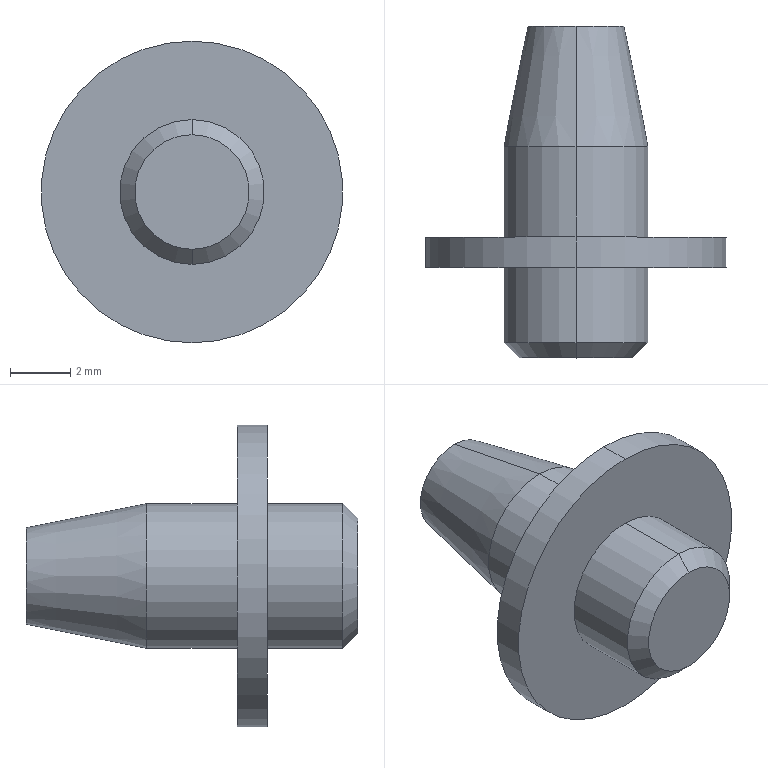Part | STEP file | TYLJ-BJ-007 Pin(1mm thick)-dddeger | 1 solid | 14 faces | box 10 x 11 x 10 mm | volume 236.295 mm3 | cylinder 6 | cone 4 | plane 4 | commonest cylinder face diameters 4.8 x4 10 x2
STEP:
#1=CARTESIAN_POINT('',(0.,0.,0.));
#2=DIRECTION('',(0.,0.,1.));
#3=DIRECTION('',(1.,0.,0.));
#4=AXIS2_PLACEMENT_3D('',#1,#2,#3);
#5=CARTESIAN_POINT('',(0.,0.,-1.9));
#6=VERTEX_POINT('',#5);
#7=CARTESIAN_POINT('',(0.,0.,1.9));
#8=VERTEX_POINT('',#7);
#9=CARTESIAN_POINT('',(0.,0.,0.));
#10=DIRECTION('',(0.,-1.,0.));
#11=DIRECTION('',(0.,0.,-1.));
#12=AXIS2_PLACEMENT_3D('',#9,#10,#11);
#13=CIRCLE('',#12,1.9);
#14=CARTESIAN_POINT('',(0.,0.,0.));
#15=DIRECTION('',(0.,1.,0.));
#16=DIRECTION('',(0.,0.,1.));
#17=AXIS2_PLACEMENT_3D('',#14,#15,#16);
#18=CONICAL_SURFACE('',#17,1.9,0.7854);
#19=CARTESIAN_POINT('',(3.142,0.));
#20=DIRECTION('',(-1.,0.));
#21=VECTOR('',#20,1.);
#22=LINE('',#19,#21);
#23=(GEOMETRIC_REPRESENTATION_CONTEXT(2)PARAMETRIC_REPRESENTATION_CONTEXT()REPRESENTATION_CONTEXT('',''));
#24=DEFINITIONAL_REPRESENTATION('',(#22),#23);
#25=PCURVE('',#18,#24);
#26=CARTESIAN_POINT('',(0.,0.,0.));
#27=DIRECTION('',(0.,-1.,0.));
#28=DIRECTION('',(0.,0.,-1.));
#29=AXIS2_PLACEMENT_3D('',#26,#27,#28);
#30=PLANE('',#29);
#31=CARTESIAN_POINT('',(0.,0.));
#32=DIRECTION('',(1.,0.));
#33=AXIS2_PLACEMENT_2D('',#31,#32);
#34=CIRCLE('',#33,1.9);
#35=(GEOMETRIC_REPRESENTATION_CONTEXT(2)PARAMETRIC_REPRESENTATION_CONTEXT()REPRESENTATION_CONTEXT('',''));
#36=DEFINITIONAL_REPRESENTATION('',(#34),#35);
#37=PCURVE('',#30,#36);
#38=SURFACE_CURVE('',#13,(#25,#37),.PCURVE_S1.);
#39=EDGE_CURVE('',#6,#8,#38,.T.);
#40=ORIENTED_EDGE('',*,*,#39,.F.);
#41=CARTESIAN_POINT('',(0.,0.5,-2.4));
#42=VERTEX_POINT('',#41);
#43=CARTESIAN_POINT('',(0.,0.,-1.9));
#44=DIRECTION('',(0.,0.7071,-0.7071));
#45=VECTOR('',#44,1.);
#46=LINE('',#43,#45);
#47=CARTESIAN_POINT('',(3.142,0.));
#48=DIRECTION('',(0.,1.));
#49=VECTOR('',#48,1.);
#50=LINE('',#47,#49);
#51=(GEOMETRIC_REPRESENTATION_CONTEXT(2)PARAMETRIC_REPRESENTATION_CONTEXT()REPRESENTATION_CONTEXT('',''));
#52=DEFINITIONAL_REPRESENTATION('',(#50),#51);
#53=PCURVE('',#18,#52);
#54=CARTESIAN_POINT('',(0.,0.,0.));
#55=DIRECTION('',(0.,1.,0.));
#56=DIRECTION('',(0.,0.,1.));
#57=AXIS2_PLACEMENT_3D('',#54,#55,#56);
#58=CONICAL_SURFACE('',#57,1.9,0.7854);
#59=CARTESIAN_POINT('',(3.142,0.));
#60=DIRECTION('',(0.,1.));
#61=VECTOR('',#60,1.);
#62=LINE('',#59,#61);
#63=(GEOMETRIC_REPRESENTATION_CONTEXT(2)PARAMETRIC_REPRESENTATION_CONTEXT()REPRESENTATION_CONTEXT('',''));
#64=DEFINITIONAL_REPRESENTATION('',(#62),#63);
#65=PCURVE('',#58,#64);
#66=SURFACE_CURVE('',#46,(#53,#65),.PCURVE_S1.);
#67=EDGE_CURVE('',#6,#42,#66,.T.);
#68=ORIENTED_EDGE('',*,*,#67,.T.);
#69=CARTESIAN_POINT('',(0.,0.5,2.4));
#70=VERTEX_POINT('',#69);
#71=CARTESIAN_POINT('',(0.,0.5,0.));
#72=DIRECTION('',(0.,1.,0.));
#73=DIRECTION('',(0.,0.,-1.));
#74=AXIS2_PLACEMENT_3D('',#71,#72,#73);
#75=CIRCLE('',#74,2.4);
#76=CARTESIAN_POINT('',(-3.142,0.5));
#77=DIRECTION('',(1.,0.));
#78=VECTOR('',#77,1.);
#79=LINE('',#76,#78);
#80=(GEOMETRIC_REPRESENTATION_CONTEXT(2)PARAMETRIC_REPRESENTATION_CONTEXT()REPRESENTATION_CONTEXT('',''));
#81=DEFINITIONAL_REPRESENTATION('',(#79),#80);
#82=PCURVE('',#18,#81);
#83=CARTESIAN_POINT('',(0.,11.,0.));
#84=DIRECTION('',(0.,-1.,0.));
#85=DIRECTION('',(0.,0.,-1.));
#86=AXIS2_PLACEMENT_3D('',#83,#84,#85);
#87=CYLINDRICAL_SURFACE('',#86,2.4);
#88=CARTESIAN_POINT('',(6.283,10.5));
#89=DIRECTION('',(-1.,0.));
#90=VECTOR('',#89,1.);
#91=LINE('',#88,#90);
#92=(GEOMETRIC_REPRESENTATION_CONTEXT(2)PARAMETRIC_REPRESENTATION_CONTEXT()REPRESENTATION_CONTEXT('',''));
#93=DEFINITIONAL_REPRESENTATION('',(#91),#92);
#94=PCURVE('',#87,#93);
#95=SURFACE_CURVE('',#75,(#82,#94),.PCURVE_S1.);
#96=EDGE_CURVE('',#70,#42,#95,.T.);
#97=ORIENTED_EDGE('',*,*,#96,.F.);
#98=CARTESIAN_POINT('',(0.,0.,1.9));
#99=DIRECTION('',(0.,0.7071,0.7071));
#100=VECTOR('',#99,1.);
#101=LINE('',#98,#100);
#102=CARTESIAN_POINT('',(0.,0.));
#103=DIRECTION('',(0.,1.));
#104=VECTOR('',#103,1.);
#105=LINE('',#102,#104);
#106=(GEOMETRIC_REPRESENTATION_CONTEXT(2)PARAMETRIC_REPRESENTATION_CONTEXT()REPRESENTATION_CONTEXT('',''));
#107=DEFINITIONAL_REPRESENTATION('',(#105),#106);
#108=PCURVE('',#18,#107);
#109=CARTESIAN_POINT('',(6.283,0.));
#110=DIRECTION('',(0.,1.));
#111=VECTOR('',#110,1.);
#112=LINE('',#109,#111);
#113=(GEOMETRIC_REPRESENTATION_CONTEXT(2)PARAMETRIC_REPRESENTATION_CONTEXT()REPRESENTATION_CONTEXT('',''));
#114=DEFINITIONAL_REPRESENTATION('',(#112),#113);
#115=PCURVE('',#58,#114);
#116=SURFACE_CURVE('',#101,(#108,#115),.PCURVE_S1.);
#117=EDGE_CURVE('',#8,#70,#116,.T.);
#118=ORIENTED_EDGE('',*,*,#117,.F.);
#119=EDGE_LOOP('',(#40,#68,#97,#118));
#120=FACE_BOUND('',#119,.T.);
#121=ADVANCED_FACE('',(#120),#18,.T.);
#122=CARTESIAN_POINT('',(0.,7.,-2.4));
#123=VERTEX_POINT('',#122);
#124=CARTESIAN_POINT('',(0.,7.,2.4));
#125=VERTEX_POINT('',#124);
#126=CARTESIAN_POINT('',(0.,7.,0.));
#127=DIRECTION('',(0.,-1.,0.));
#128=DIRECTION('',(0.,0.,-1.));
#129=AXIS2_PLACEMENT_3D('',#126,#127,#128);
#130=CIRCLE('',#129,2.4);
#131=CARTESIAN_POINT('',(0.,11.,0.));
#132=DIRECTION('',(0.,-1.,0.));
#133=DIRECTION('',(0.,0.,-1.));
#134=AXIS2_PLACEMENT_3D('',#131,#132,#133);
#135=CYLINDRICAL_SURFACE('',#134,2.4);
#136=CARTESIAN_POINT('',(0.,4.));
#137=DIRECTION('',(1.,0.));
#138=VECTOR('',#137,1.);
#139=LINE('',#136,#138);
#140=(GEOMETRIC_REPRESENTATION_CONTEXT(2)PARAMETRIC_REPRESENTATION_CONTEXT()REPRESENTATION_CONTEXT('',''));
#141=DEFINITIONAL_REPRESENTATION('',(#139),#140);
#142=PCURVE('',#135,#141);
#143=CARTESIAN_POINT('',(0.,7.,0.));
#144=DIRECTION('',(0.,-1.,0.));
#145=DIRECTION('',(0.,0.,-1.));
#146=AXIS2_PLACEMENT_3D('',#143,#144,#145);
#147=CONICAL_SURFACE('',#146,2.4,0.1974);
#148=CARTESIAN_POINT('',(0.,0.));
#149=DIRECTION('',(1.,0.));
#150=VECTOR('',#149,1.);
#151=LINE('',#148,#150);
#152=(GEOMETRIC_REPRESENTATION_CONTEXT(2)PARAMETRIC_REPRESENTATION_CONTEXT()REPRESENTATION_CONTEXT('',''));
#153=DEFINITIONAL_REPRESENTATION('',(#151),#152);
#154=PCURVE('',#147,#153);
#155=SURFACE_CURVE('',#130,(#142,#154),.PCURVE_S1.);
#156=EDGE_CURVE('',#123,#125,#155,.T.);
#157=ORIENTED_EDGE('',*,*,#156,.T.);
#158=CARTESIAN_POINT('',(0.,4.,2.4));
#159=VERTEX_POINT('',#158);
#160=CARTESIAN_POINT('',(0.,11.,2.4));
#161=DIRECTION('',(0.,-1.,0.));
#162=VECTOR('',#161,1.);
#163=LINE('',#160,#162);
#164=CARTESIAN_POINT('',(3.142,0.));
#165=DIRECTION('',(0.,1.));
#166=VECTOR('',#165,1.);
#167=LINE('',#164,#166);
#168=(GEOMETRIC_REPRESENTATION_CONTEXT(2)PARAMETRIC_REPRESENTATION_CONTEXT()REPRESENTATION_CONTEXT('',''));
#169=DEFINITIONAL_REPRESENTATION('',(#167),#168);
#170=PCURVE('',#135,#169);
#171=CARTESIAN_POINT('',(0.,11.,0.));
#172=DIRECTION('',(0.,-1.,0.));
#173=DIRECTION('',(0.,0.,-1.));
#174=AXIS2_PLACEMENT_3D('',#171,#172,#173);
#175=CYLINDRICAL_SURFACE('',#174,2.4);
#176=CARTESIAN_POINT('',(3.142,0.));
#177=DIRECTION('',(0.,1.));
#178=VECTOR('',#177,1.);
#179=LINE('',#176,#178);
#180=(GEOMETRIC_REPRESENTATION_CONTEXT(2)PARAMETRIC_REPRESENTATION_CONTEXT()REPRESENTATION_CONTEXT('',''));
#181=DEFINITIONAL_REPRESENTATION('',(#179),#180);
#182=PCURVE('',#175,#181);
#183=SURFACE_CURVE('',#163,(#170,#182),.PCURVE_S1.);
#184=EDGE_CURVE('',#125,#159,#183,.T.);
#185=ORIENTED_EDGE('',*,*,#184,.T.);
#186=CARTESIAN_POINT('',(0.,4.,-2.4));
#187=VERTEX_POINT('',#186);
#188=CARTESIAN_POINT('',(0.,4.,0.));
#189=DIRECTION('',(0.,-1.,0.));
#190=DIRECTION('',(0.,0.,-1.));
#191=AXIS2_PLACEMENT_3D('',#188,#189,#190);
#192=CIRCLE('',#191,2.4);
#193=CARTESIAN_POINT('',(0.,7.));
#194=DIRECTION('',(1.,0.));
#195=VECTOR('',#194,1.);
#196=LINE('',#193,#195);
#197=(GEOMETRIC_REPRESENTATION_CONTEXT(2)PARAMETRIC_REPRESENTATION_CONTEXT()REPRESENTATION_CONTEXT('',''));
#198=DEFINITIONAL_REPRESENTATION('',(#196),#197);
#199=PCURVE('',#135,#198);
#200=CARTESIAN_POINT('',(5.,4.,0.));
#201=DIRECTION('',(0.,1.,0.));
#202=DIRECTION('',(0.,0.,1.));
#203=AXIS2_PLACEMENT_3D('',#200,#201,#202);
#204=PLANE('',#203);
#205=CARTESIAN_POINT('',(-2.4,-5.));
#206=CARTESIAN_POINT('',(-2.4,-0.8431));
#207=CARTESIAN_POINT('',(1.2,-2.922));
#208=CARTESIAN_POINT('',(4.8,-5.));
#209=CARTESIAN_POINT('',(1.2,-7.078));
#210=CARTESIAN_POINT('',(-2.4,-9.157));
#211=CARTESIAN_POINT('',(-2.4,-5.));
#212=(BOUNDED_CURVE()B_SPLINE_CURVE(2,(#205,#206,#207,#208,#209,#210,#211),.UNSPECIFIED.,.T.,.F.)B_SPLINE_CURVE_WITH_KNOTS((1,2,2,2,2,1),(-2.094,0.,2.094,4.189,6.283,8.378),.UNSPECIFIED.)CURVE()GEOMETRIC_REPRESENTATION_ITEM()RATIONAL_B_SPLINE_CURVE((1.,0.5,1.,0.5,1.,0.5,1.))REPRESENTATION_ITEM(''));
#213=(GEOMETRIC_REPRESENTATION_CONTEXT(2)PARAMETRIC_REPRESENTATION_CONTEXT()REPRESENTATION_CONTEXT('',''));
#214=DEFINITIONAL_REPRESENTATION('',(#212),#213);
#215=PCURVE('',#204,#214);
#216=SURFACE_CURVE('',#192,(#199,#215),.PCURVE_S1.);
#217=EDGE_CURVE('',#187,#159,#216,.T.);
#218=ORIENTED_EDGE('',*,*,#217,.F.);
#219=CARTESIAN_POINT('',(0.,11.,-2.4));
#220=DIRECTION('',(0.,-1.,0.));
#221=VECTOR('',#220,1.);
#222=LINE('',#219,#221);
#223=CARTESIAN_POINT('',(0.,0.));
#224=DIRECTION('',(0.,1.));
#225=VECTOR('',#224,1.);
#226=LINE('',#223,#225);
#227=(GEOMETRIC_REPRESENTATION_CONTEXT(2)PARAMETRIC_REPRESENTATION_CONTEXT()REPRESENTATION_CONTEXT('',''));
#228=DEFINITIONAL_REPRESENTATION('',(#226),#227);
#229=PCURVE('',#135,#228);
#230=CARTESIAN_POINT('',(6.283,0.));
#231=DIRECTION('',(0.,1.));
#232=VECTOR('',#231,1.);
#233=LINE('',#230,#232);
#234=(GEOMETRIC_REPRESENTATION_CONTEXT(2)PARAMETRIC_REPRESENTATION_CONTEXT()REPRESENTATION_CONTEXT('',''));
#235=DEFINITIONAL_REPRESENTATION('',(#233),#234);
#236=PCURVE('',#175,#235);
#237=SURFACE_CURVE('',#222,(#229,#236),.PCURVE_S1.);
#238=EDGE_CURVE('',#123,#187,#237,.T.);
#239=ORIENTED_EDGE('',*,*,#238,.F.);
#240=EDGE_LOOP('',(#157,#185,#218,#239));
#241=FACE_BOUND('',#240,.T.);
#242=ADVANCED_FACE('',(#241),#135,.T.);
#243=CARTESIAN_POINT('',(0.,4.,-5.));
#244=VERTEX_POINT('',#243);
#245=CARTESIAN_POINT('',(0.,4.,5.));
#246=VERTEX_POINT('',#245);
#247=CARTESIAN_POINT('',(0.,4.,0.));
#248=DIRECTION('',(0.,-1.,0.));
#249=DIRECTION('',(0.,0.,-1.));
#250=AXIS2_PLACEMENT_3D('',#247,#248,#249);
#251=CIRCLE('',#250,5.);
#252=CARTESIAN_POINT('',(0.,11.,0.));
#253=DIRECTION('',(0.,-1.,0.));
#254=DIRECTION('',(0.,0.,-1.));
#255=AXIS2_PLACEMENT_3D('',#252,#253,#254);
#256=CYLINDRICAL_SURFACE('',#255,5.);
#257=CARTESIAN_POINT('',(0.,7.));
#258=DIRECTION('',(1.,0.));
#259=VECTOR('',#258,1.);
#260=LINE('',#257,#259);
#261=(GEOMETRIC_REPRESENTATION_CONTEXT(2)PARAMETRIC_REPRESENTATION_CONTEXT()REPRESENTATION_CONTEXT('',''));
#262=DEFINITIONAL_REPRESENTATION('',(#260),#261);
#263=PCURVE('',#256,#262);
#264=CARTESIAN_POINT('',(-5.,-5.));
#265=CARTESIAN_POINT('',(-5.,3.66));
#266=CARTESIAN_POINT('',(2.5,-0.6699));
#267=CARTESIAN_POINT('',(10.,-5.));
#268=CARTESIAN_POINT('',(2.5,-9.33));
#269=CARTESIAN_POINT('',(-5.,-13.66));
#270=CARTESIAN_POINT('',(-5.,-5.));
#271=(BOUNDED_CURVE()B_SPLINE_CURVE(2,(#264,#265,#266,#267,#268,#269,#270),.UNSPECIFIED.,.T.,.F.)B_SPLINE_CURVE_WITH_KNOTS((1,2,2,2,2,1),(-2.094,0.,2.094,4.189,6.283,8.378),.UNSPECIFIED.)CURVE()GEOMETRIC_REPRESENTATION_ITEM()RATIONAL_B_SPLINE_CURVE((1.,0.5,1.,0.5,1.,0.5,1.))REPRESENTATION_ITEM(''));
#272=(GEOMETRIC_REPRESENTATION_CONTEXT(2)PARAMETRIC_REPRESENTATION_CONTEXT()REPRESENTATION_CONTEXT('',''));
#273=DEFINITIONAL_REPRESENTATION('',(#271),#272);
#274=PCURVE('',#204,#273);
#275=SURFACE_CURVE('',#251,(#263,#274),.PCURVE_S1.);
#276=EDGE_CURVE('',#244,#246,#275,.T.);
#277=ORIENTED_EDGE('',*,*,#276,.T.);
#278=CARTESIAN_POINT('',(0.,3.,5.));
#279=VERTEX_POINT('',#278);
#280=CARTESIAN_POINT('',(0.,11.,5.));
#281=DIRECTION('',(0.,-1.,0.));
#282=VECTOR('',#281,1.);
#283=LINE('',#280,#282);
#284=CARTESIAN_POINT('',(3.142,0.));
#285=DIRECTION('',(0.,1.));
#286=VECTOR('',#285,1.);
#287=LINE('',#284,#286);
#288=(GEOMETRIC_REPRESENTATION_CONTEXT(2)PARAMETRIC_REPRESENTATION_CONTEXT()REPRESENTATION_CONTEXT('',''));
#289=DEFINITIONAL_REPRESENTATION('',(#287),#288);
#290=PCURVE('',#256,#289);
#291=CARTESIAN_POINT('',(0.,11.,0.));
#292=DIRECTION('',(0.,-1.,0.));
#293=DIRECTION('',(0.,0.,-1.));
#294=AXIS2_PLACEMENT_3D('',#291,#292,#293);
#295=CYLINDRICAL_SURFACE('',#294,5.);
#296=CARTESIAN_POINT('',(3.142,0.));
#297=DIRECTION('',(0.,1.));
#298=VECTOR('',#297,1.);
#299=LINE('',#296,#298);
#300=(GEOMETRIC_REPRESENTATION_CONTEXT(2)PARAMETRIC_REPRESENTATION_CONTEXT()REPRESENTATION_CONTEXT('',''));
#301=DEFINITIONAL_REPRESENTATION('',(#299),#300);
#302=PCURVE('',#295,#301);
#303=SURFACE_CURVE('',#283,(#290,#302),.PCURVE_S1.);
#304=EDGE_CURVE('',#246,#279,#303,.T.);
#305=ORIENTED_EDGE('',*,*,#304,.T.);
#306=CARTESIAN_POINT('',(0.,3.,-5.));
#307=VERTEX_POINT('',#306);
#308=CARTESIAN_POINT('',(0.,3.,0.));
#309=DIRECTION('',(0.,-1.,0.));
#310=DIRECTION('',(0.,0.,-1.));
#311=AXIS2_PLACEMENT_3D('',#308,#309,#310);
#312=CIRCLE('',#311,5.);
#313=CARTESIAN_POINT('',(0.,8.));
#314=DIRECTION('',(1.,0.));
#315=VECTOR('',#314,1.);
#316=LINE('',#313,#315);
#317=(GEOMETRIC_REPRESENTATION_CONTEXT(2)PARAMETRIC_REPRESENTATION_CONTEXT()REPRESENTATION_CONTEXT('',''));
#318=DEFINITIONAL_REPRESENTATION('',(#316),#317);
#319=PCURVE('',#256,#318);
#320=CARTESIAN_POINT('',(2.4,3.,0.));
#321=DIRECTION('',(0.,-1.,0.));
#322=DIRECTION('',(0.,0.,-1.));
#323=AXIS2_PLACEMENT_3D('',#320,#321,#322);
#324=PLANE('',#323);
#325=CARTESIAN_POINT('',(0.,-2.4));
#326=DIRECTION('',(1.,0.));
#327=AXIS2_PLACEMENT_2D('',#325,#326);
#328=CIRCLE('',#327,5.);
#329=(GEOMETRIC_REPRESENTATION_CONTEXT(2)PARAMETRIC_REPRESENTATION_CONTEXT()REPRESENTATION_CONTEXT('',''));
#330=DEFINITIONAL_REPRESENTATION('',(#328),#329);
#331=PCURVE('',#324,#330);
#332=SURFACE_CURVE('',#312,(#319,#331),.PCURVE_S1.);
#333=EDGE_CURVE('',#307,#279,#332,.T.);
#334=ORIENTED_EDGE('',*,*,#333,.F.);
#335=CARTESIAN_POINT('',(0.,11.,-5.));
#336=DIRECTION('',(0.,-1.,0.));
#337=VECTOR('',#336,1.);
#338=LINE('',#335,#337);
#339=CARTESIAN_POINT('',(0.,0.));
#340=DIRECTION('',(0.,1.));
#341=VECTOR('',#340,1.);
#342=LINE('',#339,#341);
#343=(GEOMETRIC_REPRESENTATION_CONTEXT(2)PARAMETRIC_REPRESENTATION_CONTEXT()REPRESENTATION_CONTEXT('',''));
#344=DEFINITIONAL_REPRESENTATION('',(#342),#343);
#345=PCURVE('',#256,#344);
#346=CARTESIAN_POINT('',(6.283,0.));
#347=DIRECTION('',(0.,1.));
#348=VECTOR('',#347,1.);
#349=LINE('',#346,#348);
#350=(GEOMETRIC_REPRESENTATION_CONTEXT(2)PARAMETRIC_REPRESENTATION_CONTEXT()REPRESENTATION_CONTEXT('',''));
#351=DEFINITIONAL_REPRESENTATION('',(#349),#350);
#352=PCURVE('',#295,#351);
#353=SURFACE_CURVE('',#338,(#345,#352),.PCURVE_S1.);
#354=EDGE_CURVE('',#244,#307,#353,.T.);
#355=ORIENTED_EDGE('',*,*,#354,.F.);
#356=EDGE_LOOP('',(#277,#305,#334,#355));
#357=FACE_BOUND('',#356,.T.);
#358=ADVANCED_FACE('',(#357),#256,.T.);
#359=CARTESIAN_POINT('',(0.,3.,-2.4));
#360=VERTEX_POINT('',#359);
#361=CARTESIAN_POINT('',(0.,3.,2.4));
#362=VERTEX_POINT('',#361);
#363=CARTESIAN_POINT('',(0.,3.,0.));
#364=DIRECTION('',(0.,-1.,0.));
#365=DIRECTION('',(0.,0.,-1.));
#366=AXIS2_PLACEMENT_3D('',#363,#364,#365);
#367=CIRCLE('',#366,2.4);
#368=CARTESIAN_POINT('',(0.,8.));
#369=DIRECTION('',(1.,0.));
#370=VECTOR('',#369,1.);
#371=LINE('',#368,#370);
#372=(GEOMETRIC_REPRESENTATION_CONTEXT(2)PARAMETRIC_REPRESENTATION_CONTEXT()REPRESENTATION_CONTEXT('',''));
#373=DEFINITIONAL_REPRESENTATION('',(#371),#372);
#374=PCURVE('',#87,#373);
#375=CARTESIAN_POINT('',(0.,-2.4));
#376=DIRECTION('',(1.,0.));
#377=AXIS2_PLACEMENT_2D('',#375,#376);
#378=CIRCLE('',#377,2.4);
#379=(GEOMETRIC_REPRESENTATION_CONTEXT(2)PARAMETRIC_REPRESENTATION_CONTEXT()REPRESENTATION_CONTEXT('',''));
#380=DEFINITIONAL_REPRESENTATION('',(#378),#379);
#381=PCURVE('',#324,#380);
#382=SURFACE_CURVE('',#367,(#374,#381),.PCURVE_S1.);
#383=EDGE_CURVE('',#360,#362,#382,.T.);
#384=ORIENTED_EDGE('',*,*,#383,.T.);
#385=CARTESIAN_POINT('',(0.,11.,2.4));
#386=DIRECTION('',(0.,-1.,0.));
#387=VECTOR('',#386,1.);
#388=LINE('',#385,#387);
#389=CARTESIAN_POINT('',(3.142,0.));
#390=DIRECTION('',(0.,1.));
#391=VECTOR('',#390,1.);
#392=LINE('',#389,#391);
#393=(GEOMETRIC_REPRESENTATION_CONTEXT(2)PARAMETRIC_REPRESENTATION_CONTEXT()REPRESENTATION_CONTEXT('',''));
#394=DEFINITIONAL_REPRESENTATION('',(#392),#393);
#395=PCURVE('',#87,#394);
#396=CARTESIAN_POINT('',(0.,11.,0.));
#397=DIRECTION('',(0.,-1.,0.));
#398=DIRECTION('',(0.,0.,-1.));
#399=AXIS2_PLACEMENT_3D('',#396,#397,#398);
#400=CYLINDRICAL_SURFACE('',#399,2.4);
#401=CARTESIAN_POINT('',(3.142,0.));
#402=DIRECTION('',(0.,1.));
#403=VECTOR('',#402,1.);
#404=LINE('',#401,#403);
#405=(GEOMETRIC_REPRESENTATION_CONTEXT(2)PARAMETRIC_REPRESENTATION_CONTEXT()REPRESENTATION_CONTEXT('',''));
#406=DEFINITIONAL_REPRESENTATION('',(#404),#405);
#407=PCURVE('',#400,#406);
#408=SURFACE_CURVE('',#388,(#395,#407),.PCURVE_S1.);
#409=EDGE_CURVE('',#362,#70,#408,.T.);
#410=ORIENTED_EDGE('',*,*,#409,.T.);
#411=ORIENTED_EDGE('',*,*,#96,.T.);
#412=CARTESIAN_POINT('',(0.,11.,-2.4));
#413=DIRECTION('',(0.,-1.,0.));
#414=VECTOR('',#413,1.);
#415=LINE('',#412,#414);
#416=CARTESIAN_POINT('',(0.,0.));
#417=DIRECTION('',(0.,1.));
#418=VECTOR('',#417,1.);
#419=LINE('',#416,#418);
#420=(GEOMETRIC_REPRESENTATION_CONTEXT(2)PARAMETRIC_REPRESENTATION_CONTEXT()REPRESENTATION_CONTEXT('',''));
#421=DEFINITIONAL_REPRESENTATION('',(#419),#420);
#422=PCURVE('',#87,#421);
#423=CARTESIAN_POINT('',(6.283,0.));
#424=DIRECTION('',(0.,1.));
#425=VECTOR('',#424,1.);
#426=LINE('',#423,#425);
#427=(GEOMETRIC_REPRESENTATION_CONTEXT(2)PARAMETRIC_REPRESENTATION_CONTEXT()REPRESENTATION_CONTEXT('',''));
#428=DEFINITIONAL_REPRESENTATION('',(#426),#427);
#429=PCURVE('',#400,#428);
#430=SURFACE_CURVE('',#415,(#422,#429),.PCURVE_S1.);
#431=EDGE_CURVE('',#360,#42,#430,.T.);
#432=ORIENTED_EDGE('',*,*,#431,.F.);
#433=EDGE_LOOP('',(#384,#410,#411,#432));
#434=FACE_BOUND('',#433,.T.);
#435=ADVANCED_FACE('',(#434),#87,.T.);
#436=CARTESIAN_POINT('',(0.,11.,-1.6));
#437=VERTEX_POINT('',#436);
#438=CARTESIAN_POINT('',(0.,11.,1.6));
#439=VERTEX_POINT('',#438);
#440=CARTESIAN_POINT('',(0.,11.,0.));
#441=DIRECTION('',(0.,-1.,0.));
#442=DIRECTION('',(0.,0.,-1.));
#443=AXIS2_PLACEMENT_3D('',#440,#441,#442);
#444=CIRCLE('',#443,1.6);
#445=CARTESIAN_POINT('',(0.,-4.));
#446=DIRECTION('',(1.,0.));
#447=VECTOR('',#446,1.);
#448=LINE('',#445,#447);
#449=(GEOMETRIC_REPRESENTATION_CONTEXT(2)PARAMETRIC_REPRESENTATION_CONTEXT()REPRESENTATION_CONTEXT('',''));
#450=DEFINITIONAL_REPRESENTATION('',(#448),#449);
#451=PCURVE('',#147,#450);
#452=CARTESIAN_POINT('',(1.6,11.,0.));
#453=DIRECTION('',(0.,1.,0.));
#454=DIRECTION('',(0.,0.,1.));
#455=AXIS2_PLACEMENT_3D('',#452,#453,#454);
#456=PLANE('',#455);
#457=CARTESIAN_POINT('',(-1.6,-1.6));
#458=CARTESIAN_POINT('',(-1.6,1.171));
#459=CARTESIAN_POINT('',(0.8,-0.2144));
#460=CARTESIAN_POINT('',(3.2,-1.6));
#461=CARTESIAN_POINT('',(0.8,-2.986));
#462=CARTESIAN_POINT('',(-1.6,-4.371));
#463=CARTESIAN_POINT('',(-1.6,-1.6));
#464=(BOUNDED_CURVE()B_SPLINE_CURVE(2,(#457,#458,#459,#460,#461,#462,#463),.UNSPECIFIED.,.T.,.F.)B_SPLINE_CURVE_WITH_KNOTS((1,2,2,2,2,1),(-2.094,0.,2.094,4.189,6.283,8.378),.UNSPECIFIED.)CURVE()GEOMETRIC_REPRESENTATION_ITEM()RATIONAL_B_SPLINE_CURVE((1.,0.5,1.,0.5,1.,0.5,1.))REPRESENTATION_ITEM(''));
#465=(GEOMETRIC_REPRESENTATION_CONTEXT(2)PARAMETRIC_REPRESENTATION_CONTEXT()REPRESENTATION_CONTEXT('',''));
#466=DEFINITIONAL_REPRESENTATION('',(#464),#465);
#467=PCURVE('',#456,#466);
#468=SURFACE_CURVE('',#444,(#451,#467),.PCURVE_S1.);
#469=EDGE_CURVE('',#437,#439,#468,.T.);
#470=ORIENTED_EDGE('',*,*,#469,.T.);
#471=CARTESIAN_POINT('',(0.,7.,2.4));
#472=DIRECTION('',(0.,-0.9806,0.1961));
#473=VECTOR('',#472,1.);
#474=LINE('',#471,#473);
#475=CARTESIAN_POINT('',(3.142,0.));
#476=DIRECTION('',(0.,1.));
#477=VECTOR('',#476,1.);
#478=LINE('',#475,#477);
#479=(GEOMETRIC_REPRESENTATION_CONTEXT(2)PARAMETRIC_REPRESENTATION_CONTEXT()REPRESENTATION_CONTEXT('',''));
#480=DEFINITIONAL_REPRESENTATION('',(#478),#479);
#481=PCURVE('',#147,#480);
#482=CARTESIAN_POINT('',(0.,7.,0.));
#483=DIRECTION('',(0.,-1.,0.));
#484=DIRECTION('',(0.,0.,-1.));
#485=AXIS2_PLACEMENT_3D('',#482,#483,#484);
#486=CONICAL_SURFACE('',#485,2.4,0.1974);
#487=CARTESIAN_POINT('',(3.142,0.));
#488=DIRECTION('',(0.,1.));
#489=VECTOR('',#488,1.);
#490=LINE('',#487,#489);
#491=(GEOMETRIC_REPRESENTATION_CONTEXT(2)PARAMETRIC_REPRESENTATION_CONTEXT()REPRESENTATION_CONTEXT('',''));
#492=DEFINITIONAL_REPRESENTATION('',(#490),#491);
#493=PCURVE('',#486,#492);
#494=SURFACE_CURVE('',#474,(#481,#493),.PCURVE_S1.);
#495=EDGE_CURVE('',#439,#125,#494,.T.);
#496=ORIENTED_EDGE('',*,*,#495,.T.);
#497=ORIENTED_EDGE('',*,*,#156,.F.);
#498=CARTESIAN_POINT('',(0.,7.,-2.4));
#499=DIRECTION('',(0.,-0.9806,-0.1961));
#500=VECTOR('',#499,1.);
#501=LINE('',#498,#500);
#502=CARTESIAN_POINT('',(0.,0.));
#503=DIRECTION('',(0.,1.));
#504=VECTOR('',#503,1.);
#505=LINE('',#502,#504);
#506=(GEOMETRIC_REPRESENTATION_CONTEXT(2)PARAMETRIC_REPRESENTATION_CONTEXT()REPRESENTATION_CONTEXT('',''));
#507=DEFINITIONAL_REPRESENTATION('',(#505),#506);
#508=PCURVE('',#147,#507);
#509=CARTESIAN_POINT('',(6.283,0.));
#510=DIRECTION('',(0.,1.));
#511=VECTOR('',#510,1.);
#512=LINE('',#509,#511);
#513=(GEOMETRIC_REPRESENTATION_CONTEXT(2)PARAMETRIC_REPRESENTATION_CONTEXT()REPRESENTATION_CONTEXT('',''));
#514=DEFINITIONAL_REPRESENTATION('',(#512),#513);
#515=PCURVE('',#486,#514);
#516=SURFACE_CURVE('',#501,(#508,#515),.PCURVE_S1.);
#517=EDGE_CURVE('',#437,#123,#516,.T.);
#518=ORIENTED_EDGE('',*,*,#517,.F.);
#519=EDGE_LOOP('',(#470,#496,#497,#518));
#520=FACE_BOUND('',#519,.T.);
#521=ADVANCED_FACE('',(#520),#147,.T.);
#522=ORIENTED_EDGE('',*,*,#495,.F.);
#523=CARTESIAN_POINT('',(0.,11.,0.));
#524=DIRECTION('',(0.,-1.,0.));
#525=DIRECTION('',(0.,0.,-1.));
#526=AXIS2_PLACEMENT_3D('',#523,#524,#525);
#527=CIRCLE('',#526,1.6);
#528=CARTESIAN_POINT('',(0.,-4.));
#529=DIRECTION('',(1.,0.));
#530=VECTOR('',#529,1.);
#531=LINE('',#528,#530);
#532=(GEOMETRIC_REPRESENTATION_CONTEXT(2)PARAMETRIC_REPRESENTATION_CONTEXT()REPRESENTATION_CONTEXT('',''));
#533=DEFINITIONAL_REPRESENTATION('',(#531),#532);
#534=PCURVE('',#486,#533);
#535=CARTESIAN_POINT('',(-1.6,-1.6));
#536=CARTESIAN_POINT('',(-1.6,1.171));
#537=CARTESIAN_POINT('',(0.8,-0.2144));
#538=CARTESIAN_POINT('',(3.2,-1.6));
#539=CARTESIAN_POINT('',(0.8,-2.986));
#540=CARTESIAN_POINT('',(-1.6,-4.371));
#541=CARTESIAN_POINT('',(-1.6,-1.6));
#542=(BOUNDED_CURVE()B_SPLINE_CURVE(2,(#535,#536,#537,#538,#539,#540,#541),.UNSPECIFIED.,.T.,.F.)B_SPLINE_CURVE_WITH_KNOTS((1,2,2,2,2,1),(-2.094,0.,2.094,4.189,6.283,8.378),.UNSPECIFIED.)CURVE()GEOMETRIC_REPRESENTATION_ITEM()RATIONAL_B_SPLINE_CURVE((1.,0.5,1.,0.5,1.,0.5,1.))REPRESENTATION_ITEM(''));
#543=(GEOMETRIC_REPRESENTATION_CONTEXT(2)PARAMETRIC_REPRESENTATION_CONTEXT()REPRESENTATION_CONTEXT('',''));
#544=DEFINITIONAL_REPRESENTATION('',(#542),#543);
#545=PCURVE('',#456,#544);
#546=SURFACE_CURVE('',#527,(#534,#545),.PCURVE_S1.);
#547=EDGE_CURVE('',#439,#437,#546,.T.);
#548=ORIENTED_EDGE('',*,*,#547,.T.);
#549=ORIENTED_EDGE('',*,*,#517,.T.);
#550=CARTESIAN_POINT('',(0.,7.,0.));
#551=DIRECTION('',(0.,-1.,0.));
#552=DIRECTION('',(0.,0.,-1.));
#553=AXIS2_PLACEMENT_3D('',#550,#551,#552);
#554=CIRCLE('',#553,2.4);
#555=CARTESIAN_POINT('',(0.,0.));
#556=DIRECTION('',(1.,0.));
#557=VECTOR('',#556,1.);
#558=LINE('',#555,#557);
#559=(GEOMETRIC_REPRESENTATION_CONTEXT(2)PARAMETRIC_REPRESENTATION_CONTEXT()REPRESENTATION_CONTEXT('',''));
#560=DEFINITIONAL_REPRESENTATION('',(#558),#559);
#561=PCURVE('',#486,#560);
#562=CARTESIAN_POINT('',(0.,4.));
#563=DIRECTION('',(1.,0.));
#564=VECTOR('',#563,1.);
#565=LINE('',#562,#564);
#566=(GEOMETRIC_REPRESENTATION_CONTEXT(2)PARAMETRIC_REPRESENTATION_CONTEXT()REPRESENTATION_CONTEXT('',''));
#567=DEFINITIONAL_REPRESENTATION('',(#565),#566);
#568=PCURVE('',#175,#567);
#569=SURFACE_CURVE('',#554,(#561,#568),.PCURVE_S1.);
#570=EDGE_CURVE('',#125,#123,#569,.T.);
#571=ORIENTED_EDGE('',*,*,#570,.F.);
#572=EDGE_LOOP('',(#522,#548,#549,#571));
#573=FACE_BOUND('',#572,.T.);
#574=ADVANCED_FACE('',(#573),#486,.T.);
#575=ORIENTED_EDGE('',*,*,#469,.F.);
#576=ORIENTED_EDGE('',*,*,#547,.F.);
#577=EDGE_LOOP('',(#575,#576));
#578=FACE_BOUND('',#577,.T.);
#579=ADVANCED_FACE('',(#578),#456,.T.);
#580=CARTESIAN_POINT('',(0.,0.,0.));
#581=DIRECTION('',(0.,-1.,0.));
#582=DIRECTION('',(0.,0.,-1.));
#583=AXIS2_PLACEMENT_3D('',#580,#581,#582);
#584=CIRCLE('',#583,1.9);
#585=CARTESIAN_POINT('',(0.,0.));
#586=DIRECTION('',(1.,0.));
#587=AXIS2_PLACEMENT_2D('',#585,#586);
#588=CIRCLE('',#587,1.9);
#589=(GEOMETRIC_REPRESENTATION_CONTEXT(2)PARAMETRIC_REPRESENTATION_CONTEXT()REPRESENTATION_CONTEXT('',''));
#590=DEFINITIONAL_REPRESENTATION('',(#588),#589);
#591=PCURVE('',#30,#590);
#592=CARTESIAN_POINT('',(9.425,0.));
#593=DIRECTION('',(-1.,0.));
#594=VECTOR('',#593,1.);
#595=LINE('',#592,#594);
#596=(GEOMETRIC_REPRESENTATION_CONTEXT(2)PARAMETRIC_REPRESENTATION_CONTEXT()REPRESENTATION_CONTEXT('',''));
#597=DEFINITIONAL_REPRESENTATION('',(#595),#596);
#598=PCURVE('',#58,#597);
#599=SURFACE_CURVE('',#584,(#591,#598),.PCURVE_S1.);
#600=EDGE_CURVE('',#8,#6,#599,.T.);
#601=ORIENTED_EDGE('',*,*,#600,.T.);
#602=ORIENTED_EDGE('',*,*,#39,.T.);
#603=EDGE_LOOP('',(#601,#602));
#604=FACE_BOUND('',#603,.T.);
#605=ADVANCED_FACE('',(#604),#30,.T.);
#606=ORIENTED_EDGE('',*,*,#409,.F.);
#607=CARTESIAN_POINT('',(0.,3.,0.));
#608=DIRECTION('',(0.,-1.,0.));
#609=DIRECTION('',(0.,0.,-1.));
#610=AXIS2_PLACEMENT_3D('',#607,#608,#609);
#611=CIRCLE('',#610,2.4);
#612=CARTESIAN_POINT('',(0.,8.));
#613=DIRECTION('',(1.,0.));
#614=VECTOR('',#613,1.);
#615=LINE('',#612,#614);
#616=(GEOMETRIC_REPRESENTATION_CONTEXT(2)PARAMETRIC_REPRESENTATION_CONTEXT()REPRESENTATION_CONTEXT('',''));
#617=DEFINITIONAL_REPRESENTATION('',(#615),#616);
#618=PCURVE('',#400,#617);
#619=CARTESIAN_POINT('',(0.,-2.4));
#620=DIRECTION('',(1.,0.));
#621=AXIS2_PLACEMENT_2D('',#619,#620);
#622=CIRCLE('',#621,2.4);
#623=(GEOMETRIC_REPRESENTATION_CONTEXT(2)PARAMETRIC_REPRESENTATION_CONTEXT()REPRESENTATION_CONTEXT('',''));
#624=DEFINITIONAL_REPRESENTATION('',(#622),#623);
#625=PCURVE('',#324,#624);
#626=SURFACE_CURVE('',#611,(#618,#625),.PCURVE_S1.);
#627=EDGE_CURVE('',#362,#360,#626,.T.);
#628=ORIENTED_EDGE('',*,*,#627,.T.);
#629=ORIENTED_EDGE('',*,*,#431,.T.);
#630=CARTESIAN_POINT('',(0.,0.5,0.));
#631=DIRECTION('',(0.,1.,0.));
#632=DIRECTION('',(0.,0.,-1.));
#633=AXIS2_PLACEMENT_3D('',#630,#631,#632);
#634=CIRCLE('',#633,2.4);
#635=CARTESIAN_POINT('',(6.283,10.5));
#636=DIRECTION('',(-1.,0.));
#637=VECTOR('',#636,1.);
#638=LINE('',#635,#637);
#639=(GEOMETRIC_REPRESENTATION_CONTEXT(2)PARAMETRIC_REPRESENTATION_CONTEXT()REPRESENTATION_CONTEXT('',''));
#640=DEFINITIONAL_REPRESENTATION('',(#638),#639);
#641=PCURVE('',#400,#640);
#642=CARTESIAN_POINT('',(3.142,0.5));
#643=DIRECTION('',(1.,0.));
#644=VECTOR('',#643,1.);
#645=LINE('',#642,#644);
#646=(GEOMETRIC_REPRESENTATION_CONTEXT(2)PARAMETRIC_REPRESENTATION_CONTEXT()REPRESENTATION_CONTEXT('',''));
#647=DEFINITIONAL_REPRESENTATION('',(#645),#646);
#648=PCURVE('',#58,#647);
#649=SURFACE_CURVE('',#634,(#641,#648),.PCURVE_S1.);
#650=EDGE_CURVE('',#42,#70,#649,.T.);
#651=ORIENTED_EDGE('',*,*,#650,.T.);
#652=EDGE_LOOP('',(#606,#628,#629,#651));
#653=FACE_BOUND('',#652,.T.);
#654=ADVANCED_FACE('',(#653),#400,.T.);
#655=ORIENTED_EDGE('',*,*,#333,.T.);
#656=CARTESIAN_POINT('',(0.,3.,0.));
#657=DIRECTION('',(0.,-1.,0.));
#658=DIRECTION('',(0.,0.,-1.));
#659=AXIS2_PLACEMENT_3D('',#656,#657,#658);
#660=CIRCLE('',#659,5.);
#661=CARTESIAN_POINT('',(0.,-2.4));
#662=DIRECTION('',(1.,0.));
#663=AXIS2_PLACEMENT_2D('',#661,#662);
#664=CIRCLE('',#663,5.);
#665=(GEOMETRIC_REPRESENTATION_CONTEXT(2)PARAMETRIC_REPRESENTATION_CONTEXT()REPRESENTATION_CONTEXT('',''));
#666=DEFINITIONAL_REPRESENTATION('',(#664),#665);
#667=PCURVE('',#324,#666);
#668=CARTESIAN_POINT('',(0.,8.));
#669=DIRECTION('',(1.,0.));
#670=VECTOR('',#669,1.);
#671=LINE('',#668,#670);
#672=(GEOMETRIC_REPRESENTATION_CONTEXT(2)PARAMETRIC_REPRESENTATION_CONTEXT()REPRESENTATION_CONTEXT('',''));
#673=DEFINITIONAL_REPRESENTATION('',(#671),#672);
#674=PCURVE('',#295,#673);
#675=SURFACE_CURVE('',#660,(#667,#674),.PCURVE_S1.);
#676=EDGE_CURVE('',#279,#307,#675,.T.);
#677=ORIENTED_EDGE('',*,*,#676,.T.);
#678=EDGE_LOOP('',(#655,#677));
#679=FACE_BOUND('',#678,.T.);
#680=ORIENTED_EDGE('',*,*,#383,.F.);
#681=ORIENTED_EDGE('',*,*,#627,.F.);
#682=EDGE_LOOP('',(#680,#681));
#683=FACE_BOUND('',#682,.T.);
#684=ADVANCED_FACE('',(#679,#683),#324,.T.);
#685=ORIENTED_EDGE('',*,*,#304,.F.);
#686=CARTESIAN_POINT('',(0.,4.,0.));
#687=DIRECTION('',(0.,-1.,0.));
#688=DIRECTION('',(0.,0.,-1.));
#689=AXIS2_PLACEMENT_3D('',#686,#687,#688);
#690=CIRCLE('',#689,5.);
#691=CARTESIAN_POINT('',(0.,7.));
#692=DIRECTION('',(1.,0.));
#693=VECTOR('',#692,1.);
#694=LINE('',#691,#693);
#695=(GEOMETRIC_REPRESENTATION_CONTEXT(2)PARAMETRIC_REPRESENTATION_CONTEXT()REPRESENTATION_CONTEXT('',''));
#696=DEFINITIONAL_REPRESENTATION('',(#694),#695);
#697=PCURVE('',#295,#696);
#698=CARTESIAN_POINT('',(-5.,-5.));
#699=CARTESIAN_POINT('',(-5.,3.66));
#700=CARTESIAN_POINT('',(2.5,-0.6699));
#701=CARTESIAN_POINT('',(10.,-5.));
#702=CARTESIAN_POINT('',(2.5,-9.33));
#703=CARTESIAN_POINT('',(-5.,-13.66));
#704=CARTESIAN_POINT('',(-5.,-5.));
#705=(BOUNDED_CURVE()B_SPLINE_CURVE(2,(#698,#699,#700,#701,#702,#703,#704),.UNSPECIFIED.,.T.,.F.)B_SPLINE_CURVE_WITH_KNOTS((1,2,2,2,2,1),(-2.094,0.,2.094,4.189,6.283,8.378),.UNSPECIFIED.)CURVE()GEOMETRIC_REPRESENTATION_ITEM()RATIONAL_B_SPLINE_CURVE((1.,0.5,1.,0.5,1.,0.5,1.))REPRESENTATION_ITEM(''));
#706=(GEOMETRIC_REPRESENTATION_CONTEXT(2)PARAMETRIC_REPRESENTATION_CONTEXT()REPRESENTATION_CONTEXT('',''));
#707=DEFINITIONAL_REPRESENTATION('',(#705),#706);
#708=PCURVE('',#204,#707);
#709=SURFACE_CURVE('',#690,(#697,#708),.PCURVE_S1.);
#710=EDGE_CURVE('',#246,#244,#709,.T.);
#711=ORIENTED_EDGE('',*,*,#710,.T.);
#712=ORIENTED_EDGE('',*,*,#354,.T.);
#713=ORIENTED_EDGE('',*,*,#676,.F.);
#714=EDGE_LOOP('',(#685,#711,#712,#713));
#715=FACE_BOUND('',#714,.T.);
#716=ADVANCED_FACE('',(#715),#295,.T.);
#717=ORIENTED_EDGE('',*,*,#217,.T.);
#718=CARTESIAN_POINT('',(0.,4.,0.));
#719=DIRECTION('',(0.,-1.,0.));
#720=DIRECTION('',(0.,0.,-1.));
#721=AXIS2_PLACEMENT_3D('',#718,#719,#720);
#722=CIRCLE('',#721,2.4);
#723=CARTESIAN_POINT('',(-2.4,-5.));
#724=CARTESIAN_POINT('',(-2.4,-0.8431));
#725=CARTESIAN_POINT('',(1.2,-2.922));
#726=CARTESIAN_POINT('',(4.8,-5.));
#727=CARTESIAN_POINT('',(1.2,-7.078));
#728=CARTESIAN_POINT('',(-2.4,-9.157));
#729=CARTESIAN_POINT('',(-2.4,-5.));
#730=(BOUNDED_CURVE()B_SPLINE_CURVE(2,(#723,#724,#725,#726,#727,#728,#729),.UNSPECIFIED.,.T.,.F.)B_SPLINE_CURVE_WITH_KNOTS((1,2,2,2,2,1),(-2.094,0.,2.094,4.189,6.283,8.378),.UNSPECIFIED.)CURVE()GEOMETRIC_REPRESENTATION_ITEM()RATIONAL_B_SPLINE_CURVE((1.,0.5,1.,0.5,1.,0.5,1.))REPRESENTATION_ITEM(''));
#731=(GEOMETRIC_REPRESENTATION_CONTEXT(2)PARAMETRIC_REPRESENTATION_CONTEXT()REPRESENTATION_CONTEXT('',''));
#732=DEFINITIONAL_REPRESENTATION('',(#730),#731);
#733=PCURVE('',#204,#732);
#734=CARTESIAN_POINT('',(0.,7.));
#735=DIRECTION('',(1.,0.));
#736=VECTOR('',#735,1.);
#737=LINE('',#734,#736);
#738=(GEOMETRIC_REPRESENTATION_CONTEXT(2)PARAMETRIC_REPRESENTATION_CONTEXT()REPRESENTATION_CONTEXT('',''));
#739=DEFINITIONAL_REPRESENTATION('',(#737),#738);
#740=PCURVE('',#175,#739);
#741=SURFACE_CURVE('',#722,(#733,#740),.PCURVE_S1.);
#742=EDGE_CURVE('',#159,#187,#741,.T.);
#743=ORIENTED_EDGE('',*,*,#742,.T.);
#744=EDGE_LOOP('',(#717,#743));
#745=FACE_BOUND('',#744,.T.);
#746=ORIENTED_EDGE('',*,*,#276,.F.);
#747=ORIENTED_EDGE('',*,*,#710,.F.);
#748=EDGE_LOOP('',(#746,#747));
#749=FACE_BOUND('',#748,.T.);
#750=ADVANCED_FACE('',(#745,#749),#204,.T.);
#751=ORIENTED_EDGE('',*,*,#184,.F.);
#752=ORIENTED_EDGE('',*,*,#570,.T.);
#753=ORIENTED_EDGE('',*,*,#238,.T.);
#754=ORIENTED_EDGE('',*,*,#742,.F.);
#755=EDGE_LOOP('',(#751,#752,#753,#754));
#756=FACE_BOUND('',#755,.T.);
#757=ADVANCED_FACE('',(#756),#175,.T.);
#758=ORIENTED_EDGE('',*,*,#67,.F.);
#759=ORIENTED_EDGE('',*,*,#600,.F.);
#760=ORIENTED_EDGE('',*,*,#117,.T.);
#761=ORIENTED_EDGE('',*,*,#650,.F.);
#762=EDGE_LOOP('',(#758,#759,#760,#761));
#763=FACE_BOUND('',#762,.T.);
#764=ADVANCED_FACE('',(#763),#58,.T.);
#765=CLOSED_SHELL('',(#121,#242,#358,#435,#521,#574,#579,#605,#654,#684,#716,#750,#757,#764));
#766=MANIFOLD_SOLID_BREP('',#765);
#767=(LENGTH_UNIT()NAMED_UNIT(*)SI_UNIT(.MILLI.,.METRE.));
#768=UNCERTAINTY_MEASURE_WITH_UNIT(LENGTH_MEASURE(0.0000001),#767,'','');
#769=(NAMED_UNIT(*)PLANE_ANGLE_UNIT()SI_UNIT($,.RADIAN.));
#770=(NAMED_UNIT(*)SI_UNIT($,.STERADIAN.)SOLID_ANGLE_UNIT());
#771=(GEOMETRIC_REPRESENTATION_CONTEXT(3)GLOBAL_UNCERTAINTY_ASSIGNED_CONTEXT((#768))GLOBAL_UNIT_ASSIGNED_CONTEXT((#767,#769,#770))REPRESENTATION_CONTEXT('',''));
#772=ADVANCED_BREP_SHAPE_REPRESENTATION('',(#4,#766),#771);